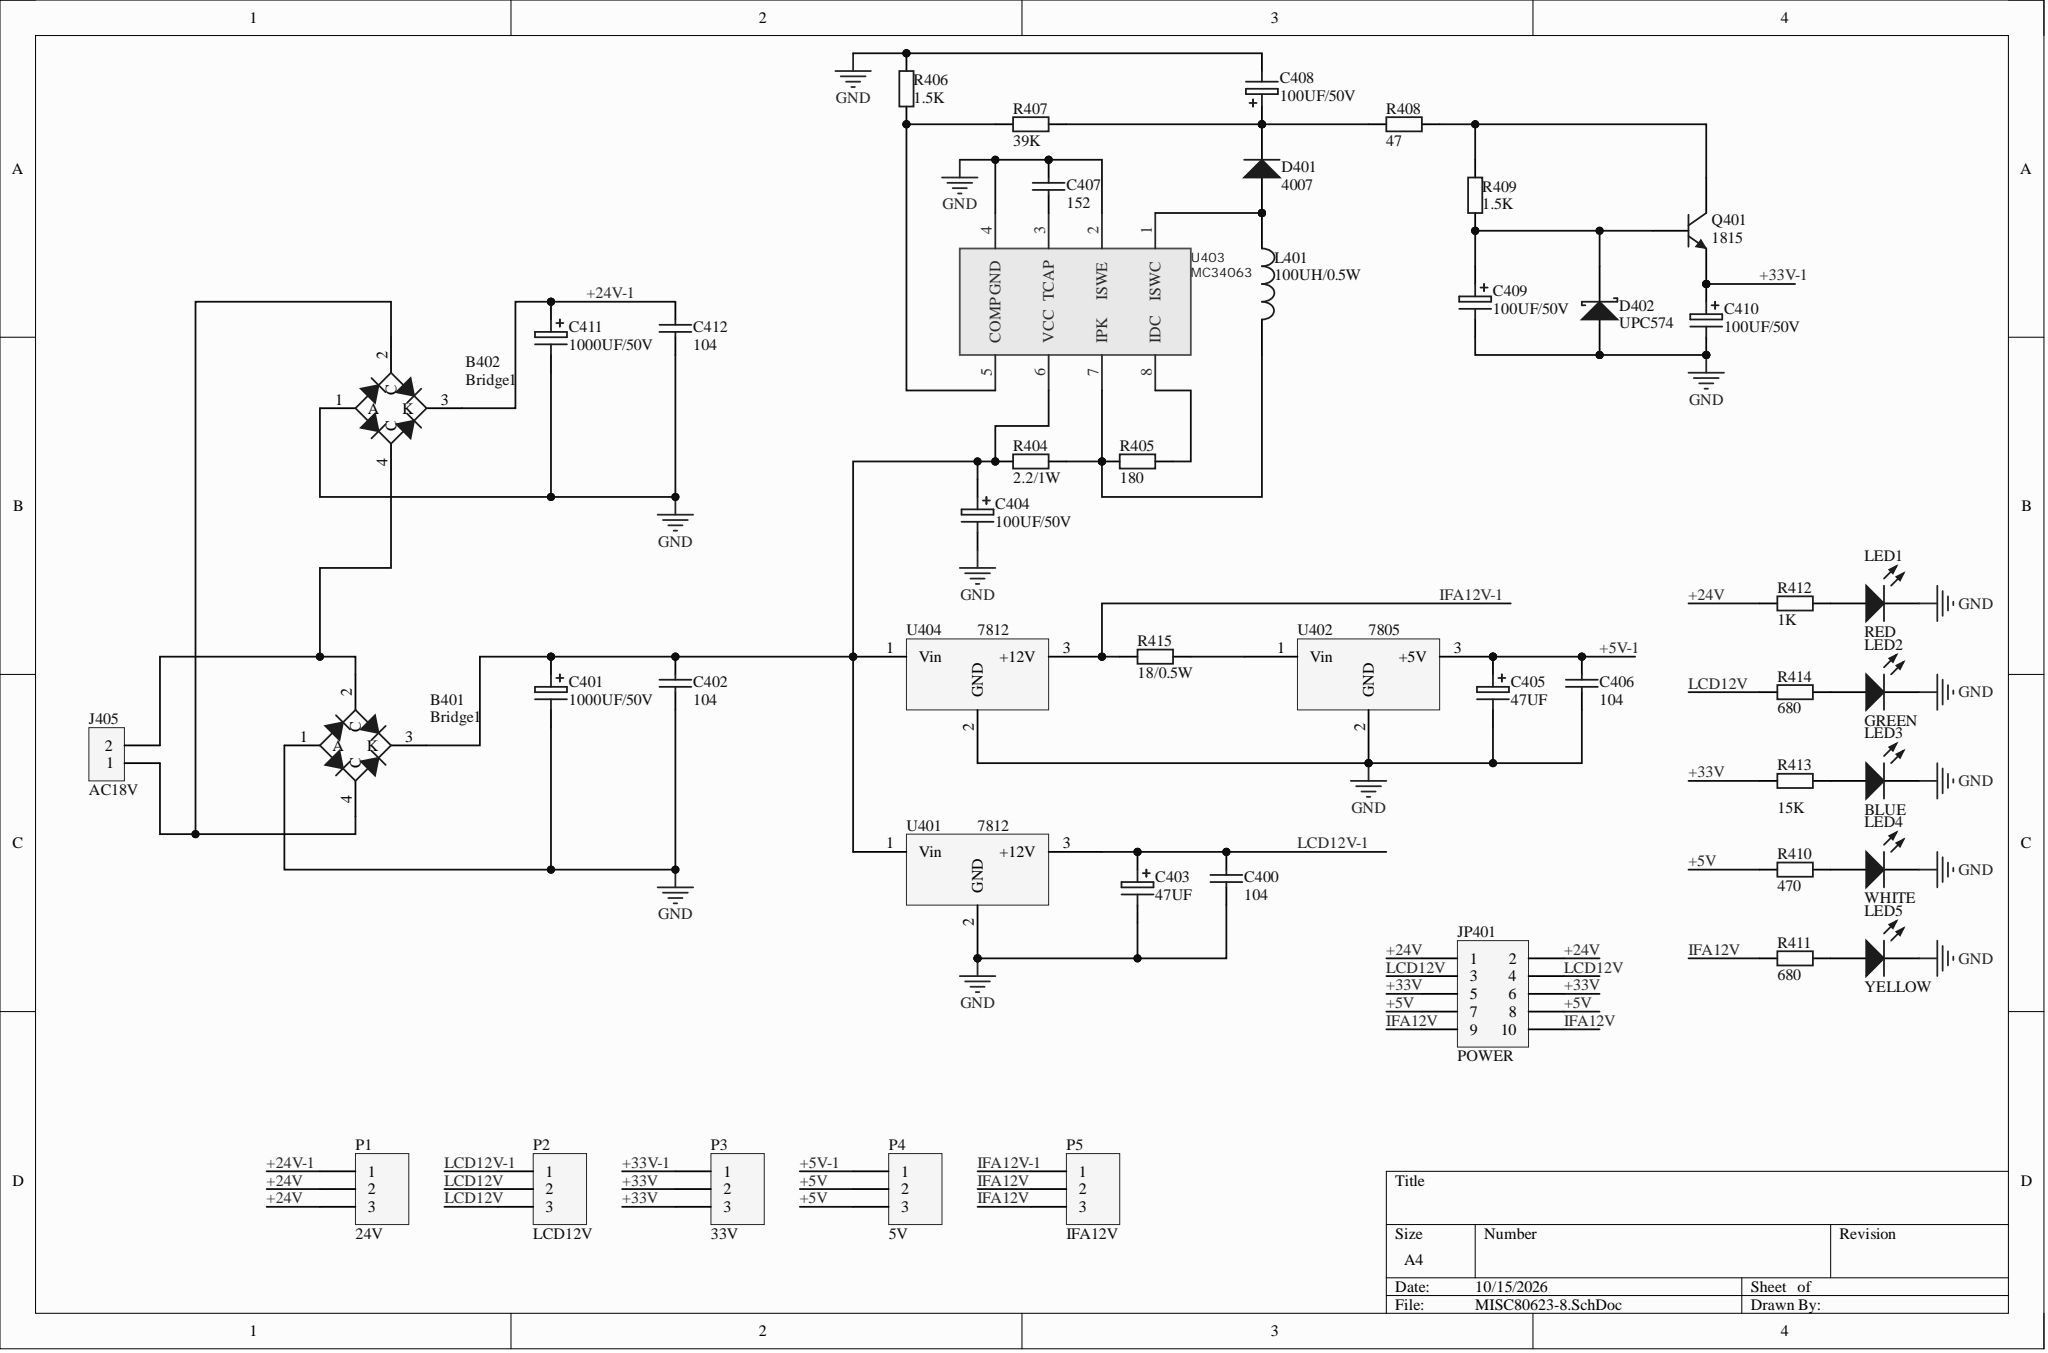Circuit board | Altium Designer | 47 parts | 28 nets
Bill of materials:
Comment,Description,Designator,Footprint,LibRef,Quantity
"Bridge1","Full Wave Diode Bridge","B401, B402","B401","Bridge1","2"
"104","","C400, C402, C406, C412","DR","CAP","4"
"1000UF/50V","","C401, C411","C401","ELECTRO1","2"
"47UF","","C403, C405","C401","ELECTRO1","2"
"100UF/50V","","C404, C408, C409, C410","C401","ELECTRO1","4"
"152","","C407","DR","CAP","1"
"4007","High Conductance Fast Diode","D401","DO-35","Diode 1N4448","1"
"UPC574","Schottky Rectifier","D402","DO-204AL","Diode 11DQ03","1"
"AC18V","Header, 2-Pin","J405","J405","Header 2","1"
"POWER","Header, 5-Pin, Dual row","JP401","JP401","Header 5X2","1"
"100UH/0.5W","INDUCTOR","L401","AL0204","INDUCTOR","1"
"RED","Typical INFRARED GaAs LED","LED1","LED","LED0","1"
"GREEN","Typical INFRARED GaAs LED","LED2","LED","LED0","1"
"BLUE","Typical INFRARED GaAs LED","LED3","LED","LED0","1"
"WHITE","Typical INFRARED GaAs LED","LED4","LED","LED0","1"
"YELLOW","Typical INFRARED GaAs LED","LED5","LED","LED0","1"
"24V","Header, 3-Pin","P1","HDR1X3","Header 3","1"
"LCD12V","Header, 3-Pin","P2","HDR1X3","Header 3","1"
"33V","Header, 3-Pin","P3","HDR1X3","Header 3","1"
"5V","Header, 3-Pin","P4","HDR1X3","Header 3","1"
"IFA12V","Header, 3-Pin","P5","HDR1X3","Header 3","1"
"1815","NPN General Purpose Amplifier","Q401","Q401","2N3904","1"
"2.2/1W","Resistor","R404","AXIAL-0.4","Res2","1"
"180","Resistor","R405","AXIAL-0.4","Res2","1"
"1.5K","Resistor","R406, R409","AXIAL-0.4","Res2","2"
"39K","Resistor","R407","AXIAL-0.4","Res2","1"
"47","Resistor","R408","AXIAL-0.4","Res2","1"
"470","Resistor","R410","AXIAL-0.4","Res2","1"
"680","Resistor","R411, R414","AXIAL-0.4","Res2","2"
"1K","Resistor","R412","AXIAL-0.4","Res2","1"
"15K","Resistor","R413","AXIAL-0.4","Res2","1"
"18/0.5W","Resistor","R415","AXIAL-0.4","Res2","1"
"7812","three-terminal voltage regulator","U401, U404","U404","AMS1117","2"
"7805","three-terminal voltage regulator","U402","U404","AMS1117","1"
"MC34063","","U403","MC34063","MC34063","1"
Netlist (Protel format):
[
B401
B401
Bridge1



]
[
B402
B401
Bridge1



]
[
C400
DR
104



]
[
C401
C401
1000UF/50V



]
[
C402
DR
104



]
[
C403
C401
47UF



]
[
C404
C401
100UF/50V



]
[
C405
C401
47UF



]
[
C406
DR
104



]
[
C407
DR
152



]
[
C408
C401
100UF/50V



]
[
C409
C401
100UF/50V



]
[
C410
C401
100UF/50V



]
[
C411
C401
1000UF/50V



]
[
C412
DR
104



]
[
D401
DO-35
4007



]
[
D402
DO-204AL
UPC574



]
[
J405
J405
AC18V



]
[
JP401
JP401
POWER



]
[
L401
AL0204
100UH/0.5W



]
[
LED1
LED
RED



]
[
LED2
LED
GREEN



]
[
LED3
LED
BLUE



]
[
LED4
LED
WHITE



]
[
LED5
LED
YELLOW



]
[
P1
HDR1X3
24V



]
[
P2
HDR1X3
LCD12V



]
[
P3
HDR1X3
33V



]
[
P4
HDR1X3
5V



]
[
P5
HDR1X3
IFA12V



]
[
Q401
Q401
1815



]
[
R404
AXIAL-0.4
2.2/1W



]
[
R405
AXIAL-0.4
180



]
[
R406
AXIAL-0.4
1.5K



]
[
R407
AXIAL-0.4
39K



]
[
R408
AXIAL-0.4
47



]
[
R409
AXIAL-0.4
1.5K



]
[
R410
AXIAL-0.4
470



]
[
R411
AXIAL-0.4
680



]
[
R412
AXIAL-0.4
1K



]
[
R413
AXIAL-0.4
15K



]
[
R414
AXIAL-0.4
680



]
[
R415
AXIAL-0.4
18/0.5W



]
[
U401
U404
7812



]
[
U402
U404
7805



]
[
U403
MC34063
MC34063



]
[
U404
U404
7812



]
(
NetR415_2
R415-2
U402-1
)
(
NetR406_1
R406-1
R407-1
U403-5
)
(
NetR405_2
R405-2
U403-8
)
(
NetQ401_3
Q401-3
R408-2
R409-2
)
(
NetLED5_1
LED5-1
R411-2
)
(
NetLED4_1
LED4-1
R410-2
)
(
NetLED3_1
LED3-1
R413-2
)
(
NetLED2_1
LED2-1
R414-2
)
(
NetLED1_1
LED1-1
R412-2
)
(
NetL401_2
L401-2
R404-2
R405-1
U403-7
)
(
NetD401_1
D401-1
L401-1
U403-1
)
(
NetC409_1
C409-1
D402-2
Q401-2
R409-1
)
(
NetC408_1
C408-1
D401-2
R407-2
R408-1
)
(
NetC407_1
C407-1
U403-3
)
(
NetB401_4
B401-4
B402-2
J405-1
)
(
NetB401_3
B401-3
C401-1
C402-2
C404-1
R404-1
U401-1
U403-6
U404-1
)
(
NetB401_2
B401-2
B402-4
J405-2
)
(
LCD12V-1
C400-2
C403-1
P2-1
U401-3
)
(
LCD12V
JP401-3
JP401-4
P2-2
P2-3
R414-1
)
(
IFA12V-1
P5-1
R415-1
U404-3
)
(
IFA12V
JP401-9
JP401-10
P5-2
P5-3
R411-1
)
(
GND
B401-1
B402-1
C400-1
C401-2
C402-1
C403-2
C404-2
C405-2
C406-1
C407-2
C408-2
C409-2
C410-2
C411-2
C412-1
D402-1
LED1-2
LED2-2
LED3-2
LED4-2
LED5-2
R406-2
U401-2
U402-2
U403-2
U403-4
U404-2
)
(
+33V-1
C410-1
P3-1
Q401-1
)
(
+33V
JP401-5
JP401-6
P3-2
P3-3
R413-1
)
(
+24V-1
B402-3
C411-1
C412-2
P1-1
)
(
+24V
JP401-1
JP401-2
P1-2
P1-3
R412-1
)
(
+5V-1
C405-1
C406-2
P4-1
U402-3
)
(
+5V
JP401-7
JP401-8
P4-2
P4-3
R410-1
)